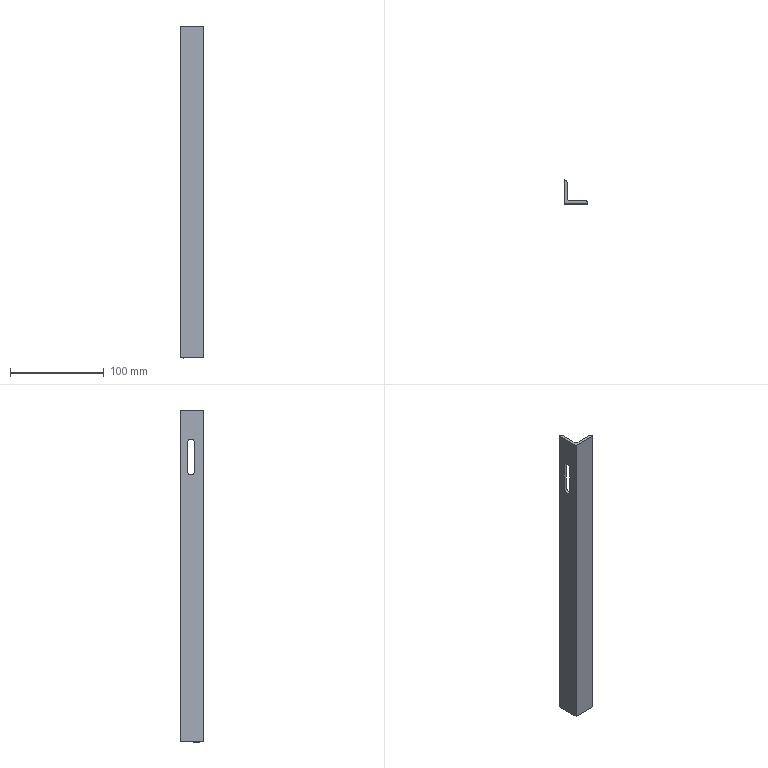Part | SolidWorks | features BaseBody 1 | 1 solid | 14 faces | box 25 x 25 x 354 mm | volume 48359 mm3 | plane 8 | cylinder 6 | commonest cylinder face diameters 6 x3 8 x3
STEP:
#1=CARTESIAN_POINT('',(3.,17.5,319.));
#2=VERTEX_POINT('',#1);
#3=CARTESIAN_POINT('',(0.,17.5,319.));
#4=VERTEX_POINT('',#3);
#5=CARTESIAN_POINT('',(10.,17.5,319.));
#6=DIRECTION('',(-1.,0.,0.));
#7=VECTOR('',#6,1000.);
#8=LINE('',#5,#7);
#9=EDGE_CURVE('',#2,#4,#8,.T.);
#10=ORIENTED_EDGE('',*,*,#9,.T.);
#11=CARTESIAN_POINT('',(0.,17.5,289.));
#12=VERTEX_POINT('',#11);
#13=CARTESIAN_POINT('',(0.,17.5,319.));
#14=DIRECTION('',(0.,0.,-1.));
#15=VECTOR('',#14,1000.);
#16=LINE('',#13,#15);
#17=EDGE_CURVE('',#4,#12,#16,.T.);
#18=ORIENTED_EDGE('',*,*,#17,.T.);
#19=CARTESIAN_POINT('',(3.,17.5,289.));
#20=VERTEX_POINT('',#19);
#21=CARTESIAN_POINT('',(10.,17.5,289.));
#22=DIRECTION('',(-1.,0.,0.));
#23=VECTOR('',#22,1000.);
#24=LINE('',#21,#23);
#25=EDGE_CURVE('',#20,#12,#24,.T.);
#26=ORIENTED_EDGE('',*,*,#25,.F.);
#27=CARTESIAN_POINT('',(3.,17.5,354.));
#28=DIRECTION('',(0.,0.,-1.));
#29=VECTOR('',#28,1000.);
#30=LINE('',#27,#29);
#31=EDGE_CURVE('',#2,#20,#30,.T.);
#32=ORIENTED_EDGE('',*,*,#31,.F.);
#33=EDGE_LOOP('',(#10,#18,#26,#32));
#34=FACE_OUTER_BOUND('',#33,.T.);
#35=CARTESIAN_POINT('',(10.,17.5,319.));
#36=DIRECTION('',(0.,1.,0.));
#37=DIRECTION('',(0.,0.,-1.));
#38=AXIS2_PLACEMENT_3D('',#35,#36,#37);
#39=PLANE('',#38);
#40=ADVANCED_FACE('',(#34),#39,.F.);
#41=ORIENTED_EDGE('',*,*,#25,.T.);
#42=CARTESIAN_POINT('',(0.,9.5,289.));
#43=VERTEX_POINT('',#42);
#44=CARTESIAN_POINT('',(0.,13.5,289.));
#45=DIRECTION('',(-1.,0.,0.));
#46=DIRECTION('',(0.,0.,1.));
#47=AXIS2_PLACEMENT_3D('',#44,#45,#46);
#48=CIRCLE('',#47,4.);
#49=EDGE_CURVE('',#12,#43,#48,.T.);
#50=ORIENTED_EDGE('',*,*,#49,.T.);
#51=CARTESIAN_POINT('',(3.,9.5,289.));
#52=VERTEX_POINT('',#51);
#53=CARTESIAN_POINT('',(10.,9.5,289.));
#54=DIRECTION('',(-1.,0.,0.));
#55=VECTOR('',#54,1000.);
#56=LINE('',#53,#55);
#57=EDGE_CURVE('',#52,#43,#56,.T.);
#58=ORIENTED_EDGE('',*,*,#57,.F.);
#59=CARTESIAN_POINT('',(3.,13.5,289.));
#60=DIRECTION('',(-1.,0.,0.));
#61=DIRECTION('',(0.,-1.,0.));
#62=AXIS2_PLACEMENT_3D('',#59,#60,#61);
#63=CIRCLE('',#62,4.);
#64=EDGE_CURVE('',#20,#52,#63,.T.);
#65=ORIENTED_EDGE('',*,*,#64,.F.);
#66=EDGE_LOOP('',(#41,#50,#58,#65));
#67=FACE_OUTER_BOUND('',#66,.T.);
#68=CARTESIAN_POINT('',(10.,13.5,289.));
#69=DIRECTION('',(-1.,0.,0.));
#70=DIRECTION('',(0.,0.,1.));
#71=AXIS2_PLACEMENT_3D('',#68,#69,#70);
#72=CYLINDRICAL_SURFACE('',#71,4.);
#73=ADVANCED_FACE('',(#67),#72,.F.);
#74=ORIENTED_EDGE('',*,*,#57,.T.);
#75=CARTESIAN_POINT('',(0.,9.5,319.));
#76=VERTEX_POINT('',#75);
#77=CARTESIAN_POINT('',(0.,9.5,319.));
#78=DIRECTION('',(0.,0.,1.));
#79=VECTOR('',#78,1000.);
#80=LINE('',#77,#79);
#81=EDGE_CURVE('',#43,#76,#80,.T.);
#82=ORIENTED_EDGE('',*,*,#81,.T.);
#83=CARTESIAN_POINT('',(3.,9.5,319.));
#84=VERTEX_POINT('',#83);
#85=CARTESIAN_POINT('',(10.,9.5,319.));
#86=DIRECTION('',(-1.,0.,0.));
#87=VECTOR('',#86,1000.);
#88=LINE('',#85,#87);
#89=EDGE_CURVE('',#84,#76,#88,.T.);
#90=ORIENTED_EDGE('',*,*,#89,.F.);
#91=CARTESIAN_POINT('',(3.,9.5,354.));
#92=DIRECTION('',(0.,0.,1.));
#93=VECTOR('',#92,1000.);
#94=LINE('',#91,#93);
#95=EDGE_CURVE('',#52,#84,#94,.T.);
#96=ORIENTED_EDGE('',*,*,#95,.F.);
#97=EDGE_LOOP('',(#74,#82,#90,#96));
#98=FACE_OUTER_BOUND('',#97,.T.);
#99=CARTESIAN_POINT('',(10.,9.5,319.));
#100=DIRECTION('',(0.,-1.,0.));
#101=DIRECTION('',(-1.,0.,0.));
#102=AXIS2_PLACEMENT_3D('',#99,#100,#101);
#103=PLANE('',#102);
#104=ADVANCED_FACE('',(#98),#103,.F.);
#105=CARTESIAN_POINT('',(3.,13.5,323.));
#106=VERTEX_POINT('',#105);
#107=CARTESIAN_POINT('',(0.,13.5,323.));
#108=VERTEX_POINT('',#107);
#109=CARTESIAN_POINT('',(10.,13.5,323.));
#110=DIRECTION('',(-1.,0.,0.));
#111=VECTOR('',#110,1000.);
#112=LINE('',#109,#111);
#113=EDGE_CURVE('',#106,#108,#112,.T.);
#114=ORIENTED_EDGE('',*,*,#113,.F.);
#115=CARTESIAN_POINT('',(3.,13.5,319.));
#116=DIRECTION('',(-1.,0.,0.));
#117=DIRECTION('',(0.,-1.,0.));
#118=AXIS2_PLACEMENT_3D('',#115,#116,#117);
#119=CIRCLE('',#118,4.);
#120=EDGE_CURVE('',#84,#106,#119,.T.);
#121=ORIENTED_EDGE('',*,*,#120,.F.);
#122=ORIENTED_EDGE('',*,*,#89,.T.);
#123=CARTESIAN_POINT('',(0.,13.5,319.));
#124=DIRECTION('',(-1.,0.,0.));
#125=DIRECTION('',(0.,0.,1.));
#126=AXIS2_PLACEMENT_3D('',#123,#124,#125);
#127=CIRCLE('',#126,4.);
#128=EDGE_CURVE('',#76,#108,#127,.T.);
#129=ORIENTED_EDGE('',*,*,#128,.T.);
#130=EDGE_LOOP('',(#114,#121,#122,#129));
#131=FACE_OUTER_BOUND('',#130,.T.);
#132=CARTESIAN_POINT('',(10.,13.5,319.));
#133=DIRECTION('',(-1.,0.,0.));
#134=DIRECTION('',(0.,0.,1.));
#135=AXIS2_PLACEMENT_3D('',#132,#133,#134);
#136=CYLINDRICAL_SURFACE('',#135,4.);
#137=ADVANCED_FACE('',(#131),#136,.F.);
#138=CARTESIAN_POINT('',(3.,22.,354.));
#139=VERTEX_POINT('',#138);
#140=CARTESIAN_POINT('',(0.,25.,354.));
#141=VERTEX_POINT('',#140);
#142=CARTESIAN_POINT('',(0.,22.,354.));
#143=DIRECTION('',(0.,0.,1.));
#144=DIRECTION('',(-1.,0.,0.));
#145=AXIS2_PLACEMENT_3D('',#142,#143,#144);
#146=CIRCLE('',#145,3.);
#147=EDGE_CURVE('',#139,#141,#146,.T.);
#148=ORIENTED_EDGE('',*,*,#147,.F.);
#149=CARTESIAN_POINT('',(3.,22.,0.));
#150=VERTEX_POINT('',#149);
#151=CARTESIAN_POINT('',(3.,22.,354.));
#152=DIRECTION('',(0.,0.,1.));
#153=VECTOR('',#152,1000.);
#154=LINE('',#151,#153);
#155=EDGE_CURVE('',#150,#139,#154,.T.);
#156=ORIENTED_EDGE('',*,*,#155,.F.);
#157=CARTESIAN_POINT('',(0.,25.,0.));
#158=VERTEX_POINT('',#157);
#159=CARTESIAN_POINT('',(0.,22.,0.));
#160=DIRECTION('',(0.,0.,-1.));
#161=DIRECTION('',(-1.,0.,0.));
#162=AXIS2_PLACEMENT_3D('',#159,#160,#161);
#163=CIRCLE('',#162,3.);
#164=EDGE_CURVE('',#158,#150,#163,.T.);
#165=ORIENTED_EDGE('',*,*,#164,.F.);
#166=CARTESIAN_POINT('',(0.,25.,354.));
#167=DIRECTION('',(0.,0.,-1.));
#168=VECTOR('',#167,1000.);
#169=LINE('',#166,#168);
#170=EDGE_CURVE('',#141,#158,#169,.T.);
#171=ORIENTED_EDGE('',*,*,#170,.F.);
#172=EDGE_LOOP('',(#148,#156,#165,#171));
#173=FACE_OUTER_BOUND('',#172,.T.);
#174=CARTESIAN_POINT('',(0.,22.,354.));
#175=DIRECTION('',(0.,0.,-1.));
#176=DIRECTION('',(-1.,0.,0.));
#177=AXIS2_PLACEMENT_3D('',#174,#175,#176);
#178=CYLINDRICAL_SURFACE('',#177,3.);
#179=ADVANCED_FACE('',(#173),#178,.T.);
#180=CARTESIAN_POINT('',(25.,0.,354.));
#181=VERTEX_POINT('',#180);
#182=CARTESIAN_POINT('',(22.,3.,354.));
#183=VERTEX_POINT('',#182);
#184=CARTESIAN_POINT('',(22.,0.,354.));
#185=DIRECTION('',(0.,0.,1.));
#186=DIRECTION('',(-1.,0.,0.));
#187=AXIS2_PLACEMENT_3D('',#184,#185,#186);
#188=CIRCLE('',#187,3.);
#189=EDGE_CURVE('',#181,#183,#188,.T.);
#190=ORIENTED_EDGE('',*,*,#189,.F.);
#191=CARTESIAN_POINT('',(25.,0.,0.));
#192=VERTEX_POINT('',#191);
#193=CARTESIAN_POINT('',(25.,0.,354.));
#194=DIRECTION('',(0.,0.,-1.));
#195=VECTOR('',#194,1000.);
#196=LINE('',#193,#195);
#197=EDGE_CURVE('',#181,#192,#196,.T.);
#198=ORIENTED_EDGE('',*,*,#197,.T.);
#199=CARTESIAN_POINT('',(22.,3.,0.));
#200=VERTEX_POINT('',#199);
#201=CARTESIAN_POINT('',(22.,0.,0.));
#202=DIRECTION('',(0.,0.,-1.));
#203=DIRECTION('',(-1.,0.,0.));
#204=AXIS2_PLACEMENT_3D('',#201,#202,#203);
#205=CIRCLE('',#204,3.);
#206=EDGE_CURVE('',#200,#192,#205,.T.);
#207=ORIENTED_EDGE('',*,*,#206,.F.);
#208=CARTESIAN_POINT('',(22.,3.,354.));
#209=DIRECTION('',(0.,0.,-1.));
#210=VECTOR('',#209,1000.);
#211=LINE('',#208,#210);
#212=EDGE_CURVE('',#183,#200,#211,.T.);
#213=ORIENTED_EDGE('',*,*,#212,.F.);
#214=EDGE_LOOP('',(#190,#198,#207,#213));
#215=FACE_OUTER_BOUND('',#214,.T.);
#216=CARTESIAN_POINT('',(22.,0.,354.));
#217=DIRECTION('',(0.,0.,-1.));
#218=DIRECTION('',(-1.,0.,0.));
#219=AXIS2_PLACEMENT_3D('',#216,#217,#218);
#220=CYLINDRICAL_SURFACE('',#219,3.);
#221=ADVANCED_FACE('',(#215),#220,.T.);
#222=CARTESIAN_POINT('',(6.,3.,354.));
#223=VERTEX_POINT('',#222);
#224=CARTESIAN_POINT('',(3.,6.,354.));
#225=VERTEX_POINT('',#224);
#226=CARTESIAN_POINT('',(6.,6.,354.));
#227=DIRECTION('',(0.,0.,-1.));
#228=DIRECTION('',(-1.,0.,0.));
#229=AXIS2_PLACEMENT_3D('',#226,#227,#228);
#230=CIRCLE('',#229,3.);
#231=EDGE_CURVE('',#223,#225,#230,.T.);
#232=ORIENTED_EDGE('',*,*,#231,.F.);
#233=CARTESIAN_POINT('',(6.,3.,0.));
#234=VERTEX_POINT('',#233);
#235=CARTESIAN_POINT('',(6.,3.,354.));
#236=DIRECTION('',(0.,0.,1.));
#237=VECTOR('',#236,1000.);
#238=LINE('',#235,#237);
#239=EDGE_CURVE('',#234,#223,#238,.T.);
#240=ORIENTED_EDGE('',*,*,#239,.F.);
#241=CARTESIAN_POINT('',(3.,6.,0.));
#242=VERTEX_POINT('',#241);
#243=CARTESIAN_POINT('',(6.,6.,0.));
#244=DIRECTION('',(0.,0.,1.));
#245=DIRECTION('',(-1.,0.,0.));
#246=AXIS2_PLACEMENT_3D('',#243,#244,#245);
#247=CIRCLE('',#246,3.);
#248=EDGE_CURVE('',#242,#234,#247,.T.);
#249=ORIENTED_EDGE('',*,*,#248,.F.);
#250=CARTESIAN_POINT('',(3.,6.,0.));
#251=DIRECTION('',(0.,0.,-1.));
#252=VECTOR('',#251,1000.);
#253=LINE('',#250,#252);
#254=EDGE_CURVE('',#225,#242,#253,.T.);
#255=ORIENTED_EDGE('',*,*,#254,.F.);
#256=EDGE_LOOP('',(#232,#240,#249,#255));
#257=FACE_OUTER_BOUND('',#256,.T.);
#258=CARTESIAN_POINT('',(6.,6.,354.));
#259=DIRECTION('',(0.,0.,1.));
#260=DIRECTION('',(1.,0.,0.));
#261=AXIS2_PLACEMENT_3D('',#258,#259,#260);
#262=CYLINDRICAL_SURFACE('',#261,3.);
#263=ADVANCED_FACE('',(#257),#262,.F.);
#264=CARTESIAN_POINT('',(3.,3.,0.));
#265=DIRECTION('',(-1.,0.,0.));
#266=VECTOR('',#265,1000.);
#267=LINE('',#264,#266);
#268=EDGE_CURVE('',#200,#234,#267,.T.);
#269=ORIENTED_EDGE('',*,*,#268,.F.);
#270=ORIENTED_EDGE('',*,*,#206,.T.);
#271=CARTESIAN_POINT('',(0.,0.,0.));
#272=VERTEX_POINT('',#271);
#273=CARTESIAN_POINT('',(0.,0.,0.));
#274=DIRECTION('',(1.,0.,0.));
#275=VECTOR('',#274,1000.);
#276=LINE('',#273,#275);
#277=EDGE_CURVE('',#272,#192,#276,.T.);
#278=ORIENTED_EDGE('',*,*,#277,.F.);
#279=CARTESIAN_POINT('',(0.,0.,0.));
#280=DIRECTION('',(0.,-1.,0.));
#281=VECTOR('',#280,1000.);
#282=LINE('',#279,#281);
#283=EDGE_CURVE('',#158,#272,#282,.T.);
#284=ORIENTED_EDGE('',*,*,#283,.F.);
#285=ORIENTED_EDGE('',*,*,#164,.T.);
#286=CARTESIAN_POINT('',(3.,25.,0.));
#287=DIRECTION('',(0.,1.,0.));
#288=VECTOR('',#287,1000.);
#289=LINE('',#286,#288);
#290=EDGE_CURVE('',#242,#150,#289,.T.);
#291=ORIENTED_EDGE('',*,*,#290,.F.);
#292=ORIENTED_EDGE('',*,*,#248,.T.);
#293=EDGE_LOOP('',(#269,#270,#278,#284,#285,#291,#292));
#294=FACE_OUTER_BOUND('',#293,.T.);
#295=CARTESIAN_POINT('',(0.,0.,0.));
#296=DIRECTION('',(0.,0.,-1.));
#297=DIRECTION('',(0.,-1.,0.));
#298=AXIS2_PLACEMENT_3D('',#295,#296,#297);
#299=PLANE('',#298);
#300=ADVANCED_FACE('',(#294),#299,.T.);
#301=CARTESIAN_POINT('',(0.,0.,354.));
#302=VERTEX_POINT('',#301);
#303=CARTESIAN_POINT('',(0.,0.,354.));
#304=DIRECTION('',(1.,0.,0.));
#305=VECTOR('',#304,1000.);
#306=LINE('',#303,#305);
#307=EDGE_CURVE('',#302,#181,#306,.T.);
#308=ORIENTED_EDGE('',*,*,#307,.T.);
#309=ORIENTED_EDGE('',*,*,#189,.T.);
#310=CARTESIAN_POINT('',(3.,3.,354.));
#311=DIRECTION('',(-1.,0.,0.));
#312=VECTOR('',#311,1000.);
#313=LINE('',#310,#312);
#314=EDGE_CURVE('',#183,#223,#313,.T.);
#315=ORIENTED_EDGE('',*,*,#314,.T.);
#316=ORIENTED_EDGE('',*,*,#231,.T.);
#317=CARTESIAN_POINT('',(3.,25.,354.));
#318=DIRECTION('',(0.,1.,0.));
#319=VECTOR('',#318,1000.);
#320=LINE('',#317,#319);
#321=EDGE_CURVE('',#225,#139,#320,.T.);
#322=ORIENTED_EDGE('',*,*,#321,.T.);
#323=ORIENTED_EDGE('',*,*,#147,.T.);
#324=CARTESIAN_POINT('',(0.,0.,354.));
#325=DIRECTION('',(0.,-1.,0.));
#326=VECTOR('',#325,1000.);
#327=LINE('',#324,#326);
#328=EDGE_CURVE('',#141,#302,#327,.T.);
#329=ORIENTED_EDGE('',*,*,#328,.T.);
#330=EDGE_LOOP('',(#308,#309,#315,#316,#322,#323,#329));
#331=FACE_OUTER_BOUND('',#330,.T.);
#332=CARTESIAN_POINT('',(0.,0.,354.));
#333=DIRECTION('',(0.,0.,-1.));
#334=DIRECTION('',(0.,-1.,0.));
#335=AXIS2_PLACEMENT_3D('',#332,#333,#334);
#336=PLANE('',#335);
#337=ADVANCED_FACE('',(#331),#336,.F.);
#338=ORIENTED_EDGE('',*,*,#95,.T.);
#339=ORIENTED_EDGE('',*,*,#120,.T.);
#340=CARTESIAN_POINT('',(3.,13.5,319.));
#341=DIRECTION('',(-1.,0.,0.));
#342=DIRECTION('',(0.,-1.,0.));
#343=AXIS2_PLACEMENT_3D('',#340,#341,#342);
#344=CIRCLE('',#343,4.);
#345=EDGE_CURVE('',#106,#2,#344,.T.);
#346=ORIENTED_EDGE('',*,*,#345,.T.);
#347=ORIENTED_EDGE('',*,*,#31,.T.);
#348=ORIENTED_EDGE('',*,*,#64,.T.);
#349=EDGE_LOOP('',(#338,#339,#346,#347,#348));
#350=FACE_BOUND('',#349,.T.);
#351=ORIENTED_EDGE('',*,*,#290,.T.);
#352=ORIENTED_EDGE('',*,*,#155,.T.);
#353=ORIENTED_EDGE('',*,*,#321,.F.);
#354=ORIENTED_EDGE('',*,*,#254,.T.);
#355=EDGE_LOOP('',(#351,#352,#353,#354));
#356=FACE_OUTER_BOUND('',#355,.T.);
#357=CARTESIAN_POINT('',(3.,25.,354.));
#358=DIRECTION('',(-1.,0.,0.));
#359=DIRECTION('',(0.,1.,0.));
#360=AXIS2_PLACEMENT_3D('',#357,#358,#359);
#361=PLANE('',#360);
#362=ADVANCED_FACE('',(#350,#356),#361,.F.);
#363=ORIENTED_EDGE('',*,*,#314,.F.);
#364=ORIENTED_EDGE('',*,*,#212,.T.);
#365=ORIENTED_EDGE('',*,*,#268,.T.);
#366=ORIENTED_EDGE('',*,*,#239,.T.);
#367=EDGE_LOOP('',(#363,#364,#365,#366));
#368=FACE_OUTER_BOUND('',#367,.T.);
#369=CARTESIAN_POINT('',(3.,3.,354.));
#370=DIRECTION('',(0.,-1.,0.));
#371=DIRECTION('',(0.,0.,-1.));
#372=AXIS2_PLACEMENT_3D('',#369,#370,#371);
#373=PLANE('',#372);
#374=ADVANCED_FACE('',(#368),#373,.F.);
#375=ORIENTED_EDGE('',*,*,#277,.T.);
#376=ORIENTED_EDGE('',*,*,#197,.F.);
#377=ORIENTED_EDGE('',*,*,#307,.F.);
#378=CARTESIAN_POINT('',(0.,0.,354.));
#379=DIRECTION('',(0.,0.,-1.));
#380=VECTOR('',#379,1000.);
#381=LINE('',#378,#380);
#382=EDGE_CURVE('',#302,#272,#381,.T.);
#383=ORIENTED_EDGE('',*,*,#382,.T.);
#384=EDGE_LOOP('',(#375,#376,#377,#383));
#385=FACE_OUTER_BOUND('',#384,.T.);
#386=CARTESIAN_POINT('',(0.,0.,354.));
#387=DIRECTION('',(0.,1.,0.));
#388=DIRECTION('',(1.,0.,0.));
#389=AXIS2_PLACEMENT_3D('',#386,#387,#388);
#390=PLANE('',#389);
#391=ADVANCED_FACE('',(#385),#390,.F.);
#392=ORIENTED_EDGE('',*,*,#17,.F.);
#393=CARTESIAN_POINT('',(0.,13.5,319.));
#394=DIRECTION('',(-1.,0.,0.));
#395=DIRECTION('',(0.,0.,1.));
#396=AXIS2_PLACEMENT_3D('',#393,#394,#395);
#397=CIRCLE('',#396,4.);
#398=EDGE_CURVE('',#108,#4,#397,.T.);
#399=ORIENTED_EDGE('',*,*,#398,.F.);
#400=ORIENTED_EDGE('',*,*,#128,.F.);
#401=ORIENTED_EDGE('',*,*,#81,.F.);
#402=ORIENTED_EDGE('',*,*,#49,.F.);
#403=EDGE_LOOP('',(#392,#399,#400,#401,#402));
#404=FACE_BOUND('',#403,.T.);
#405=ORIENTED_EDGE('',*,*,#283,.T.);
#406=ORIENTED_EDGE('',*,*,#382,.F.);
#407=ORIENTED_EDGE('',*,*,#328,.F.);
#408=ORIENTED_EDGE('',*,*,#170,.T.);
#409=EDGE_LOOP('',(#405,#406,#407,#408));
#410=FACE_OUTER_BOUND('',#409,.T.);
#411=CARTESIAN_POINT('',(0.,0.,354.));
#412=DIRECTION('',(1.,0.,0.));
#413=DIRECTION('',(0.,1.,0.));
#414=AXIS2_PLACEMENT_3D('',#411,#412,#413);
#415=PLANE('',#414);
#416=ADVANCED_FACE('',(#404,#410),#415,.F.);
#417=ORIENTED_EDGE('',*,*,#345,.F.);
#418=ORIENTED_EDGE('',*,*,#113,.T.);
#419=ORIENTED_EDGE('',*,*,#398,.T.);
#420=ORIENTED_EDGE('',*,*,#9,.F.);
#421=EDGE_LOOP('',(#417,#418,#419,#420));
#422=FACE_OUTER_BOUND('',#421,.T.);
#423=CARTESIAN_POINT('',(10.,13.5,319.));
#424=DIRECTION('',(-1.,0.,0.));
#425=DIRECTION('',(0.,0.,1.));
#426=AXIS2_PLACEMENT_3D('',#423,#424,#425);
#427=CYLINDRICAL_SURFACE('',#426,4.);
#428=ADVANCED_FACE('',(#422),#427,.F.);
#429=CLOSED_SHELL('',(#40,#73,#104,#137,#179,#221,#263,#300,#337,#362,#374,#391,#416,#428));
#430=MANIFOLD_SOLID_BREP('',#429);
#431=CARTESIAN_POINT('',(0.,0.,0.));
#432=DIRECTION('',(0.,0.,1.));
#433=DIRECTION('',(1.,0.,0.));
#434=AXIS2_PLACEMENT_3D('',#431,#432,#433);
#435=(LENGTH_UNIT()NAMED_UNIT(*)SI_UNIT(.MILLI.,.METRE.));
#436=UNCERTAINTY_MEASURE_WITH_UNIT(LENGTH_MEASURE(0.00001),#435,'','');
#437=(NAMED_UNIT(*)PLANE_ANGLE_UNIT()SI_UNIT($,.RADIAN.));
#438=(NAMED_UNIT(*)SI_UNIT($,.STERADIAN.)SOLID_ANGLE_UNIT());
#439=(GEOMETRIC_REPRESENTATION_CONTEXT(3)GLOBAL_UNCERTAINTY_ASSIGNED_CONTEXT((#436))GLOBAL_UNIT_ASSIGNED_CONTEXT((#435,#437,#438))REPRESENTATION_CONTEXT('',''));
#440=ADVANCED_BREP_SHAPE_REPRESENTATION('',(#430,#434),#439);